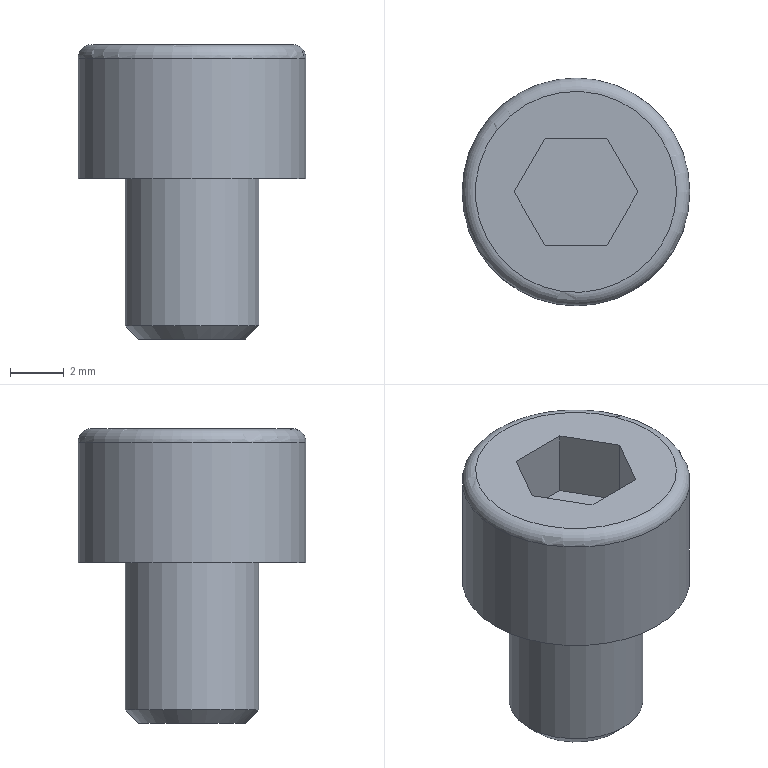Part | NX | features solid 2 | 1 solid | 14 faces | box 8.5 x 8.5 x 11 mm | volume 363.666 mm3 | plane 10 | cylinder 2 | torus 1 | cone 1 | commonest cylinder face diameters 5 x1 8.5 x1
STEP:
#1=CARTESIAN_POINT('',(175.405,-2.,-17.));
#2=VERTEX_POINT('',#1);
#3=CARTESIAN_POINT('',(176.559,0.,-17.));
#4=VERTEX_POINT('',#3);
#5=CARTESIAN_POINT('',(175.405,-2.,-17.));
#6=DIRECTION('',(0.5,0.866,0.000000992));
#7=VECTOR('',#6,1000.);
#8=LINE('',#5,#7);
#9=EDGE_CURVE('',#2,#4,#8,.T.);
#10=ORIENTED_EDGE('',*,*,#9,.F.);
#11=CARTESIAN_POINT('',(173.095,-2.,-17.));
#12=VERTEX_POINT('',#11);
#13=CARTESIAN_POINT('',(173.095,-2.,-17.));
#14=DIRECTION('',(1.,0.,0.000001984));
#15=VECTOR('',#14,1000.);
#16=LINE('',#13,#15);
#17=EDGE_CURVE('',#12,#2,#16,.T.);
#18=ORIENTED_EDGE('',*,*,#17,.F.);
#19=CARTESIAN_POINT('',(171.941,0.,-17.));
#20=VERTEX_POINT('',#19);
#21=CARTESIAN_POINT('',(171.941,0.,-17.));
#22=DIRECTION('',(0.5,-0.866,0.000000992));
#23=VECTOR('',#22,1000.);
#24=LINE('',#21,#23);
#25=EDGE_CURVE('',#20,#12,#24,.T.);
#26=ORIENTED_EDGE('',*,*,#25,.F.);
#27=CARTESIAN_POINT('',(173.095,2.,-17.));
#28=VERTEX_POINT('',#27);
#29=CARTESIAN_POINT('',(173.095,2.,-17.));
#30=DIRECTION('',(-0.5,-0.866,-0.000000992));
#31=VECTOR('',#30,1000.);
#32=LINE('',#29,#31);
#33=EDGE_CURVE('',#28,#20,#32,.T.);
#34=ORIENTED_EDGE('',*,*,#33,.F.);
#35=CARTESIAN_POINT('',(175.405,2.,-17.));
#36=VERTEX_POINT('',#35);
#37=CARTESIAN_POINT('',(175.405,2.,-17.));
#38=DIRECTION('',(-1.,0.,-0.000001984));
#39=VECTOR('',#38,1000.);
#40=LINE('',#37,#39);
#41=EDGE_CURVE('',#36,#28,#40,.T.);
#42=ORIENTED_EDGE('',*,*,#41,.F.);
#43=CARTESIAN_POINT('',(176.559,0.,-17.));
#44=DIRECTION('',(-0.5,0.866,-0.000000992));
#45=VECTOR('',#44,1000.);
#46=LINE('',#43,#45);
#47=EDGE_CURVE('',#4,#36,#46,.T.);
#48=ORIENTED_EDGE('',*,*,#47,.F.);
#49=EDGE_LOOP('',(#10,#18,#26,#34,#42,#48));
#50=FACE_BOUND('',#49,.T.);
#51=CARTESIAN_POINT('',(178.,0.,-17.));
#52=VERTEX_POINT('',#51);
#53=CARTESIAN_POINT('',(174.25,0.,-17.));
#54=DIRECTION('',(-0.000001984,0.,1.));
#55=DIRECTION('',(1.,0.,0.000001984));
#56=AXIS2_PLACEMENT_3D('',#53,#54,#55);
#57=CIRCLE('',#56,3.75);
#58=EDGE_CURVE('',#52,#52,#57,.T.);
#59=ORIENTED_EDGE('',*,*,#58,.T.);
#60=EDGE_LOOP('',(#59));
#61=FACE_BOUND('',#60,.T.);
#62=CARTESIAN_POINT('',(174.25,0.,-17.));
#63=DIRECTION('',(-0.000001984,0.,1.));
#64=DIRECTION('',(1.,0.,0.000001984));
#65=AXIS2_PLACEMENT_3D('',#62,#63,#64);
#66=PLANE('',#65);
#67=ADVANCED_FACE('',(#50,#61),#66,.T.);
#68=CARTESIAN_POINT('',(171.75,0.,-22.));
#69=VERTEX_POINT('',#68);
#70=CARTESIAN_POINT('',(174.25,0.,-22.));
#71=DIRECTION('',(0.000001984,0.,-1.));
#72=DIRECTION('',(-1.,0.,-0.000001984));
#73=AXIS2_PLACEMENT_3D('',#70,#71,#72);
#74=CIRCLE('',#73,2.5);
#75=EDGE_CURVE('',#69,#69,#74,.T.);
#76=ORIENTED_EDGE('',*,*,#75,.F.);
#77=EDGE_LOOP('',(#76));
#78=FACE_BOUND('',#77,.T.);
#79=CARTESIAN_POINT('',(178.5,0.,-22.));
#80=VERTEX_POINT('',#79);
#81=CARTESIAN_POINT('',(174.25,0.,-22.));
#82=DIRECTION('',(-0.000001984,0.,1.));
#83=DIRECTION('',(1.,0.,0.000001984));
#84=AXIS2_PLACEMENT_3D('',#81,#82,#83);
#85=CIRCLE('',#84,4.25);
#86=EDGE_CURVE('',#80,#80,#85,.T.);
#87=ORIENTED_EDGE('',*,*,#86,.F.);
#88=EDGE_LOOP('',(#87));
#89=FACE_BOUND('',#88,.T.);
#90=CARTESIAN_POINT('',(174.25,0.,-22.));
#91=DIRECTION('',(0.000001984,0.,-1.));
#92=DIRECTION('',(-1.,0.,-0.000001984));
#93=AXIS2_PLACEMENT_3D('',#90,#91,#92);
#94=PLANE('',#93);
#95=ADVANCED_FACE('',(#78,#89),#94,.T.);
#96=CARTESIAN_POINT('',(178.5,0.,-17.5));
#97=VERTEX_POINT('',#96);
#98=CARTESIAN_POINT('',(174.25,0.,-17.5));
#99=DIRECTION('',(-0.000001984,0.,1.));
#100=DIRECTION('',(1.,0.,0.000001984));
#101=AXIS2_PLACEMENT_3D('',#98,#99,#100);
#102=CIRCLE('',#101,4.25);
#103=EDGE_CURVE('',#97,#97,#102,.F.);
#104=ORIENTED_EDGE('',*,*,#103,.T.);
#105=EDGE_LOOP('',(#104));
#106=FACE_BOUND('',#105,.T.);
#107=ORIENTED_EDGE('',*,*,#86,.T.);
#108=EDGE_LOOP('',(#107));
#109=FACE_BOUND('',#108,.T.);
#110=CARTESIAN_POINT('',(174.25,0.,-22.));
#111=DIRECTION('',(-0.000001984,0.,1.));
#112=DIRECTION('',(1.,0.,0.000001984));
#113=AXIS2_PLACEMENT_3D('',#110,#111,#112);
#114=CYLINDRICAL_SURFACE('',#113,4.25);
#115=ADVANCED_FACE('',(#106,#109),#114,.T.);
#116=ORIENTED_EDGE('',*,*,#58,.F.);
#117=EDGE_LOOP('',(#116));
#118=FACE_BOUND('',#117,.T.);
#119=ORIENTED_EDGE('',*,*,#103,.F.);
#120=EDGE_LOOP('',(#119));
#121=FACE_BOUND('',#120,.T.);
#122=CARTESIAN_POINT('',(174.25,0.,-17.5));
#123=DIRECTION('',(-0.000001984,0.,1.));
#124=DIRECTION('',(1.,0.,0.000001984));
#125=AXIS2_PLACEMENT_3D('',#122,#123,#124);
#126=TOROIDAL_SURFACE('',#125,3.75,0.5);
#127=ADVANCED_FACE('',(#118,#121),#126,.T.);
#128=CARTESIAN_POINT('',(172.25,0.,-28.));
#129=VERTEX_POINT('',#128);
#130=CARTESIAN_POINT('',(174.25,0.,-28.));
#131=DIRECTION('',(0.000001984,0.,-1.));
#132=DIRECTION('',(-1.,0.,-0.000001984));
#133=AXIS2_PLACEMENT_3D('',#130,#131,#132);
#134=CIRCLE('',#133,2.);
#135=EDGE_CURVE('',#129,#129,#134,.T.);
#136=ORIENTED_EDGE('',*,*,#135,.T.);
#137=EDGE_LOOP('',(#136));
#138=FACE_BOUND('',#137,.T.);
#139=CARTESIAN_POINT('',(174.25,0.,-28.));
#140=DIRECTION('',(0.000001984,0.,-1.));
#141=DIRECTION('',(-1.,0.,-0.000001984));
#142=AXIS2_PLACEMENT_3D('',#139,#140,#141);
#143=PLANE('',#142);
#144=ADVANCED_FACE('',(#138),#143,.T.);
#145=CARTESIAN_POINT('',(171.75,0.,-27.5));
#146=VERTEX_POINT('',#145);
#147=CARTESIAN_POINT('',(174.25,0.,-27.5));
#148=DIRECTION('',(0.000001984,0.,-1.));
#149=DIRECTION('',(-1.,0.,-0.000001984));
#150=AXIS2_PLACEMENT_3D('',#147,#148,#149);
#151=CIRCLE('',#150,2.5);
#152=EDGE_CURVE('',#146,#146,#151,.F.);
#153=ORIENTED_EDGE('',*,*,#152,.T.);
#154=EDGE_LOOP('',(#153));
#155=FACE_BOUND('',#154,.T.);
#156=ORIENTED_EDGE('',*,*,#75,.T.);
#157=EDGE_LOOP('',(#156));
#158=FACE_BOUND('',#157,.T.);
#159=CARTESIAN_POINT('',(174.25,0.,-28.));
#160=DIRECTION('',(-0.000001984,0.,1.));
#161=DIRECTION('',(1.,0.,0.000001984));
#162=AXIS2_PLACEMENT_3D('',#159,#160,#161);
#163=CYLINDRICAL_SURFACE('',#162,2.5);
#164=ADVANCED_FACE('',(#155,#158),#163,.T.);
#165=ORIENTED_EDGE('',*,*,#135,.F.);
#166=EDGE_LOOP('',(#165));
#167=FACE_BOUND('',#166,.T.);
#168=ORIENTED_EDGE('',*,*,#152,.F.);
#169=EDGE_LOOP('',(#168));
#170=FACE_BOUND('',#169,.T.);
#171=CARTESIAN_POINT('',(174.25,0.,-27.5));
#172=DIRECTION('',(-0.000001984,0.,1.));
#173=DIRECTION('',(1.,0.,0.000001984));
#174=AXIS2_PLACEMENT_3D('',#171,#172,#173);
#175=CONICAL_SURFACE('',#174,2.5,0.7854);
#176=ADVANCED_FACE('',(#167,#170),#175,.T.);
#177=ORIENTED_EDGE('',*,*,#9,.T.);
#178=CARTESIAN_POINT('',(176.559,0.,-19.5));
#179=VERTEX_POINT('',#178);
#180=CARTESIAN_POINT('',(176.559,0.,-19.5));
#181=DIRECTION('',(-0.000001984,0.,1.));
#182=VECTOR('',#181,1000.);
#183=LINE('',#180,#182);
#184=EDGE_CURVE('',#179,#4,#183,.T.);
#185=ORIENTED_EDGE('',*,*,#184,.F.);
#186=CARTESIAN_POINT('',(175.405,-2.,-19.5));
#187=VERTEX_POINT('',#186);
#188=CARTESIAN_POINT('',(175.405,-2.,-19.5));
#189=DIRECTION('',(0.5,0.866,0.000000992));
#190=VECTOR('',#189,1000.);
#191=LINE('',#188,#190);
#192=EDGE_CURVE('',#187,#179,#191,.T.);
#193=ORIENTED_EDGE('',*,*,#192,.F.);
#194=CARTESIAN_POINT('',(175.405,-2.,-19.5));
#195=DIRECTION('',(-0.000001984,0.,1.));
#196=VECTOR('',#195,1000.);
#197=LINE('',#194,#196);
#198=EDGE_CURVE('',#187,#2,#197,.T.);
#199=ORIENTED_EDGE('',*,*,#198,.T.);
#200=EDGE_LOOP('',(#177,#185,#193,#199));
#201=FACE_BOUND('',#200,.T.);
#202=CARTESIAN_POINT('',(175.982,-1.,-18.25));
#203=DIRECTION('',(0.866,-0.5,0.000001718));
#204=DIRECTION('',(0.5,0.866,0.));
#205=AXIS2_PLACEMENT_3D('',#202,#203,#204);
#206=PLANE('',#205);
#207=ADVANCED_FACE('',(#201),#206,.F.);
#208=ORIENTED_EDGE('',*,*,#17,.T.);
#209=ORIENTED_EDGE('',*,*,#198,.F.);
#210=CARTESIAN_POINT('',(173.095,-2.,-19.5));
#211=VERTEX_POINT('',#210);
#212=CARTESIAN_POINT('',(173.095,-2.,-19.5));
#213=DIRECTION('',(1.,0.,0.000001984));
#214=VECTOR('',#213,1000.);
#215=LINE('',#212,#214);
#216=EDGE_CURVE('',#211,#187,#215,.T.);
#217=ORIENTED_EDGE('',*,*,#216,.F.);
#218=CARTESIAN_POINT('',(173.095,-2.,-19.5));
#219=DIRECTION('',(-0.000001984,0.,1.));
#220=VECTOR('',#219,1000.);
#221=LINE('',#218,#220);
#222=EDGE_CURVE('',#211,#12,#221,.T.);
#223=ORIENTED_EDGE('',*,*,#222,.T.);
#224=EDGE_LOOP('',(#208,#209,#217,#223));
#225=FACE_BOUND('',#224,.T.);
#226=CARTESIAN_POINT('',(174.25,-2.,-18.25));
#227=DIRECTION('',(0.,-1.,0.));
#228=DIRECTION('',(1.,0.,0.));
#229=AXIS2_PLACEMENT_3D('',#226,#227,#228);
#230=PLANE('',#229);
#231=ADVANCED_FACE('',(#225),#230,.F.);
#232=ORIENTED_EDGE('',*,*,#25,.T.);
#233=ORIENTED_EDGE('',*,*,#222,.F.);
#234=CARTESIAN_POINT('',(171.941,0.,-19.5));
#235=VERTEX_POINT('',#234);
#236=CARTESIAN_POINT('',(171.941,0.,-19.5));
#237=DIRECTION('',(0.5,-0.866,0.000000992));
#238=VECTOR('',#237,1000.);
#239=LINE('',#236,#238);
#240=EDGE_CURVE('',#235,#211,#239,.T.);
#241=ORIENTED_EDGE('',*,*,#240,.F.);
#242=CARTESIAN_POINT('',(171.941,0.,-19.5));
#243=DIRECTION('',(-0.000001984,0.,1.));
#244=VECTOR('',#243,1000.);
#245=LINE('',#242,#244);
#246=EDGE_CURVE('',#235,#20,#245,.T.);
#247=ORIENTED_EDGE('',*,*,#246,.T.);
#248=EDGE_LOOP('',(#232,#233,#241,#247));
#249=FACE_BOUND('',#248,.T.);
#250=CARTESIAN_POINT('',(172.518,-1.,-18.25));
#251=DIRECTION('',(-0.866,-0.5,-0.000001718));
#252=DIRECTION('',(0.5,-0.866,0.));
#253=AXIS2_PLACEMENT_3D('',#250,#251,#252);
#254=PLANE('',#253);
#255=ADVANCED_FACE('',(#249),#254,.F.);
#256=ORIENTED_EDGE('',*,*,#33,.T.);
#257=ORIENTED_EDGE('',*,*,#246,.F.);
#258=CARTESIAN_POINT('',(173.095,2.,-19.5));
#259=VERTEX_POINT('',#258);
#260=CARTESIAN_POINT('',(173.095,2.,-19.5));
#261=DIRECTION('',(-0.5,-0.866,-0.000000992));
#262=VECTOR('',#261,1000.);
#263=LINE('',#260,#262);
#264=EDGE_CURVE('',#259,#235,#263,.T.);
#265=ORIENTED_EDGE('',*,*,#264,.F.);
#266=CARTESIAN_POINT('',(173.095,2.,-19.5));
#267=DIRECTION('',(-0.000001984,0.,1.));
#268=VECTOR('',#267,1000.);
#269=LINE('',#266,#268);
#270=EDGE_CURVE('',#259,#28,#269,.T.);
#271=ORIENTED_EDGE('',*,*,#270,.T.);
#272=EDGE_LOOP('',(#256,#257,#265,#271));
#273=FACE_BOUND('',#272,.T.);
#274=CARTESIAN_POINT('',(172.518,1.,-18.25));
#275=DIRECTION('',(-0.866,0.5,-0.000001718));
#276=DIRECTION('',(-0.5,-0.866,0.));
#277=AXIS2_PLACEMENT_3D('',#274,#275,#276);
#278=PLANE('',#277);
#279=ADVANCED_FACE('',(#273),#278,.F.);
#280=ORIENTED_EDGE('',*,*,#41,.T.);
#281=ORIENTED_EDGE('',*,*,#270,.F.);
#282=CARTESIAN_POINT('',(175.405,2.,-19.5));
#283=VERTEX_POINT('',#282);
#284=CARTESIAN_POINT('',(175.405,2.,-19.5));
#285=DIRECTION('',(-1.,0.,-0.000001984));
#286=VECTOR('',#285,1000.);
#287=LINE('',#284,#286);
#288=EDGE_CURVE('',#283,#259,#287,.T.);
#289=ORIENTED_EDGE('',*,*,#288,.F.);
#290=CARTESIAN_POINT('',(175.405,2.,-19.5));
#291=DIRECTION('',(-0.000001984,0.,1.));
#292=VECTOR('',#291,1000.);
#293=LINE('',#290,#292);
#294=EDGE_CURVE('',#283,#36,#293,.T.);
#295=ORIENTED_EDGE('',*,*,#294,.T.);
#296=EDGE_LOOP('',(#280,#281,#289,#295));
#297=FACE_BOUND('',#296,.T.);
#298=CARTESIAN_POINT('',(174.25,2.,-18.25));
#299=DIRECTION('',(0.,1.,0.));
#300=DIRECTION('',(-1.,0.,0.));
#301=AXIS2_PLACEMENT_3D('',#298,#299,#300);
#302=PLANE('',#301);
#303=ADVANCED_FACE('',(#297),#302,.F.);
#304=ORIENTED_EDGE('',*,*,#47,.T.);
#305=ORIENTED_EDGE('',*,*,#294,.F.);
#306=CARTESIAN_POINT('',(176.559,0.,-19.5));
#307=DIRECTION('',(-0.5,0.866,-0.000000992));
#308=VECTOR('',#307,1000.);
#309=LINE('',#306,#308);
#310=EDGE_CURVE('',#179,#283,#309,.T.);
#311=ORIENTED_EDGE('',*,*,#310,.F.);
#312=ORIENTED_EDGE('',*,*,#184,.T.);
#313=EDGE_LOOP('',(#304,#305,#311,#312));
#314=FACE_BOUND('',#313,.T.);
#315=CARTESIAN_POINT('',(175.982,1.,-18.25));
#316=DIRECTION('',(0.866,0.5,0.000001718));
#317=DIRECTION('',(-0.5,0.866,0.));
#318=AXIS2_PLACEMENT_3D('',#315,#316,#317);
#319=PLANE('',#318);
#320=ADVANCED_FACE('',(#314),#319,.F.);
#321=ORIENTED_EDGE('',*,*,#310,.T.);
#322=ORIENTED_EDGE('',*,*,#288,.T.);
#323=ORIENTED_EDGE('',*,*,#264,.T.);
#324=ORIENTED_EDGE('',*,*,#240,.T.);
#325=ORIENTED_EDGE('',*,*,#216,.T.);
#326=ORIENTED_EDGE('',*,*,#192,.T.);
#327=EDGE_LOOP('',(#321,#322,#323,#324,#325,#326));
#328=FACE_BOUND('',#327,.T.);
#329=CARTESIAN_POINT('',(174.25,0.,-19.5));
#330=DIRECTION('',(0.000001984,0.,-1.));
#331=DIRECTION('',(-1.,0.,-0.000001984));
#332=AXIS2_PLACEMENT_3D('',#329,#330,#331);
#333=PLANE('',#332);
#334=ADVANCED_FACE('',(#328),#333,.F.);
#335=CLOSED_SHELL('',(#67,#95,#115,#127,#144,#164,#176,#207,#231,#255,#279,#303,#320,#334));
#336=MANIFOLD_SOLID_BREP('',#335);
#337=(LENGTH_UNIT()NAMED_UNIT(*)SI_UNIT(.MILLI.,.METRE.));
#338=UNCERTAINTY_MEASURE_WITH_UNIT(LENGTH_MEASURE(0.00001),#337,'','');
#339=(NAMED_UNIT(*)PLANE_ANGLE_UNIT()SI_UNIT($,.RADIAN.));
#340=(NAMED_UNIT(*)SI_UNIT($,.STERADIAN.)SOLID_ANGLE_UNIT());
#341=(GEOMETRIC_REPRESENTATION_CONTEXT(3)GLOBAL_UNCERTAINTY_ASSIGNED_CONTEXT((#338))GLOBAL_UNIT_ASSIGNED_CONTEXT((#337,#339,#340))REPRESENTATION_CONTEXT('',''));
#342=ADVANCED_BREP_SHAPE_REPRESENTATION('',(#336),#341);